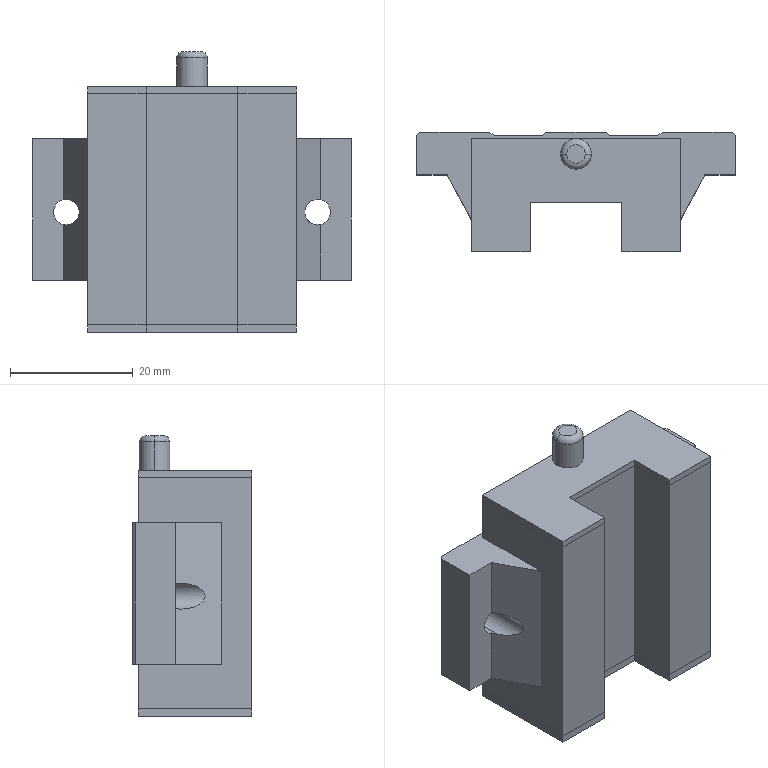Part | STEP file | Mount electronic clip sEGW15SA | 1 solid | 55 faces | box 52 x 19.5 x 45.8 mm | volume 24435 mm3 | plane 47 | cylinder 6 | torus 2 | commonest cylinder face diameters 4.2 x4 5 x2